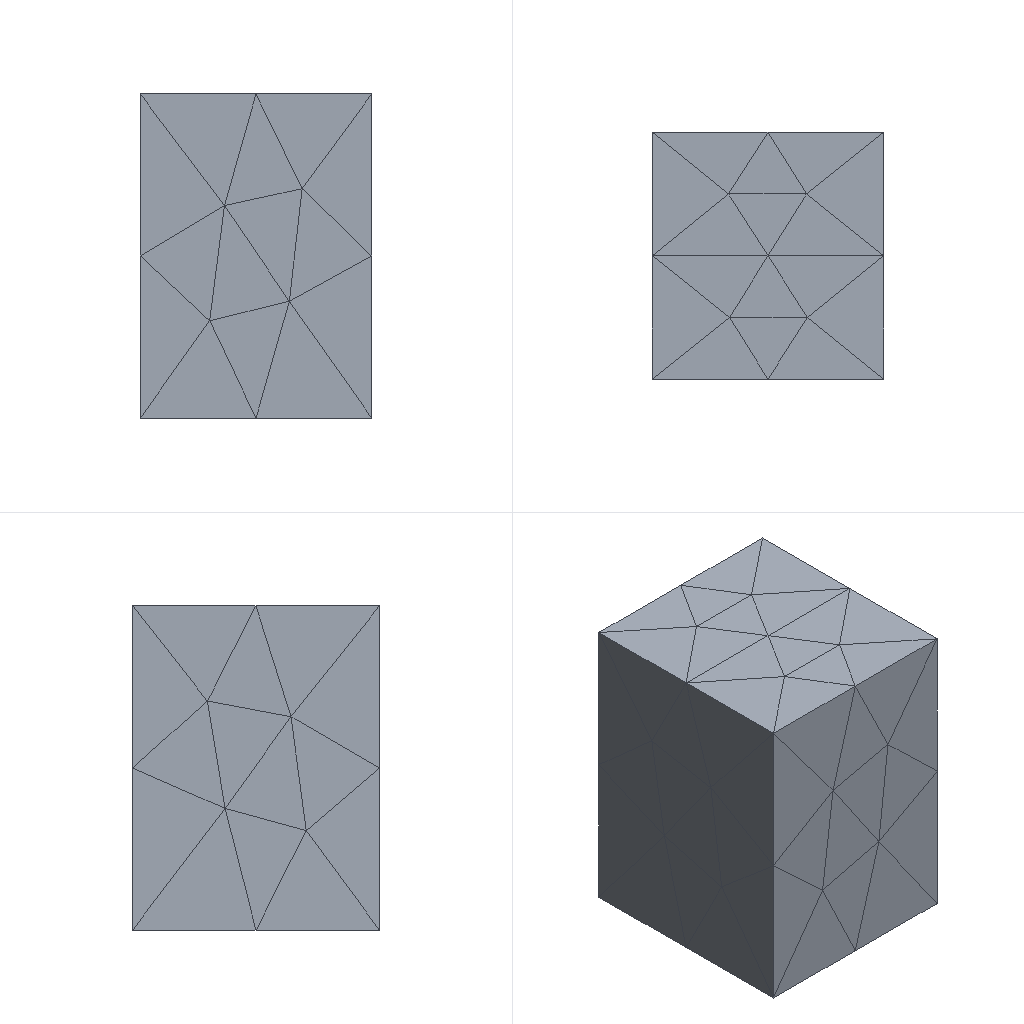Simulation study | ansys mapdl
Set-up summary:
category,name,step,type,value,unit,region
solver,ansys_mapdl
units,mm-N-s-tonne (MPa),,inferred,E=210000 density=
analysis,model,,static
mesh,nodes,,,252
mesh,elements,,,113
element_type,SOLID187,,,113
material,mat 1,,E,210000
material,mat 1,,nu,0.3
load,,model,body load temp,,,all
load,,model,force,"1000 [dir=(0, 0, -1) n=74]",,node list
bc,,model,fixed,"[dofs=UX,UY,UZ n=325]",,node list
Ansys APDL input file, long lists of numbers shortened:
/COM,ANSYS RELEASE 2026 R1           BUILD 26.1      UP20260202       09:10:51
/PREP7
/NOPR
/TITLE,2
ANTYPE, 0
*IF,_CDRDOFF,EQ,1,THEN     !if solid model was read in
_CDRDOFF=             !reset flag, numoffs already performed
*ELSE              !offset database for the following FE model
NUMOFF,NODE,      252
NUMOFF,ELEM,      113
NUMOFF,MAT ,        1
NUMOFF,TYPE,        1
*ENDIF
*SET,_RETURN ,  0.
*SET,_STATUS ,  0.
*SET,_UIQR   ,  74.
*SET,__FLOATPARAMETER__,  252.
DOF,DELETE
ETBLOCK,        1,        1
(2i9,19a9)
        1      187        0        0        0        0        0        0        0        0        0        0        0        0        0        0        0        0        0        0        0
       -1
NBLOCK,6,SOLID,       252,       252
(3i9,6e21.13e3)
        1        0        0-6.4000000000000E+001 8.0000000000000E+000
! (251 more lines like these left out)
N,UNBL,LOC,       -1,
EBLOCK,19,SOLID,       113,       113
(19i10)
         1         1         1         1         0         0         0         0        10         0         1       157        78       179       180       181       182       183       184
! (225 more lines like these left out)
        -1
MPTEMP,UNBL, 1, 1,  0.    ,
MPDATA,UNBL, 1,EX  ,       1, 1,  210000.000    ,
MPTEMP,UNBL, 1, 1,  0.    ,
MPDATA,UNBL, 1,NUXY,       1, 1, 0.3    ,
MPTEMP,UNBL, 1, 1,  0.    ,
MPDATA,UNBL, 1,PRXY,       1, 1, 0.3    ,
EXTOPT,ATTR,      0,      0,      0
EXTOPT,ESIZE,  0,  0.
EXTOPT,ACLEAR,      0
TREF,  0.
IRLF,  0
BFUNIF,TEMP,_TINY
ACEL,  0.    ,  0.    ,  0.
OMEGA,  0.    ,  0.    ,  0.
DOMEGA,  0.    ,  0.    ,  0.
CGLOC,  0.    ,  0.    ,  0.
CGOMEGA,  0.    ,  0.    ,  0.
DCGOMG,  0.    ,  0.    ,  0.
KUSE,     0
TIME,  0.
ALPHAD,  0.
BETAD,  0.
DMPRAT,  0.
DMPSTR,  0.
CRPLIM, 0.1    ,   0
CRPLIM,  0.    ,   1
NCNV,     0, 1.000000000E+12,     0,  0.    ,  0.
NEQIT,     0
ERESX,DEFA
DBLOCK,       325
(i9,a6,2(pg16.9))
        1  UX    0.00000000      0.00000000
! (324 more lines like these left out)
       -1
FBLOCK,        74
(i9,a6,2(pg16.9))
       42  FZ   -13.5135135      0.00000000
! (73 more lines like these left out)
       -1
/GO
FINISH
Results summary:
result,analysis_type_db,,,static,unstated
result,n_sets,,,1,unstated
result,load_steps[0].set,load_step=1,,1,unstated
result,load_steps[0].substep,load_step=1,,1,unstated
result,load_steps[0].time,load_step=1,,1,unstated
result,load_steps[0].freq,load_step=1,,1,unstated
result,load_steps[0].max_usum,load_step=1,,0.0004343,unstated
result,load_steps[0].max_seqv,load_step=1,,6.105,unstated
result,load_steps[0].reaction_sum.FX,load_step=1,,-1.7053e-13,unstated
result,load_steps[0].reaction_sum.FY,load_step=1,,-1.43698e-11,unstated
result,load_steps[0].reaction_sum.FZ,load_step=1,,1000,unstated
result,load_steps[0].reaction_sum.MX,load_step=1,,0,unstated
result,load_steps[0].reaction_sum.MY,load_step=1,,0,unstated
result,load_steps[0].reaction_sum.MZ,load_step=1,,0,unstated
result,convergence,,,results present for all listed sets,unstated